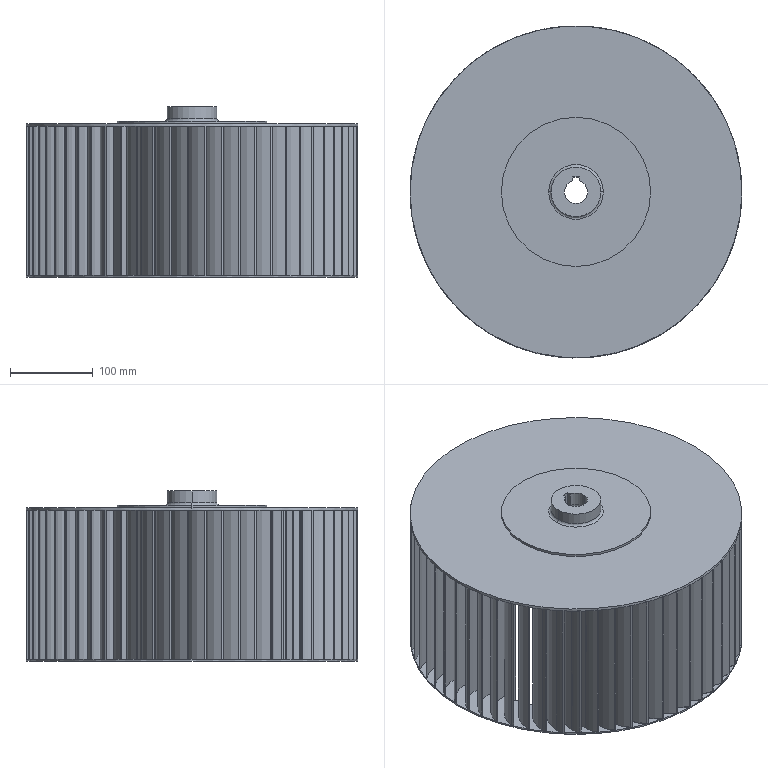Part | STEP file | Produce dryer line heating fan-SIROCCOFAN-3KW-ROLLER | 1 solid | 365 faces | box 400 x 400 x 205 mm | volume 1898819 mm3 | plane 189 | cylinder 172 | cone 2 | torus 2 | commonest cylinder face diameters 80 x150 28 x12 400 x4 60 x2 180 x2 300 x2